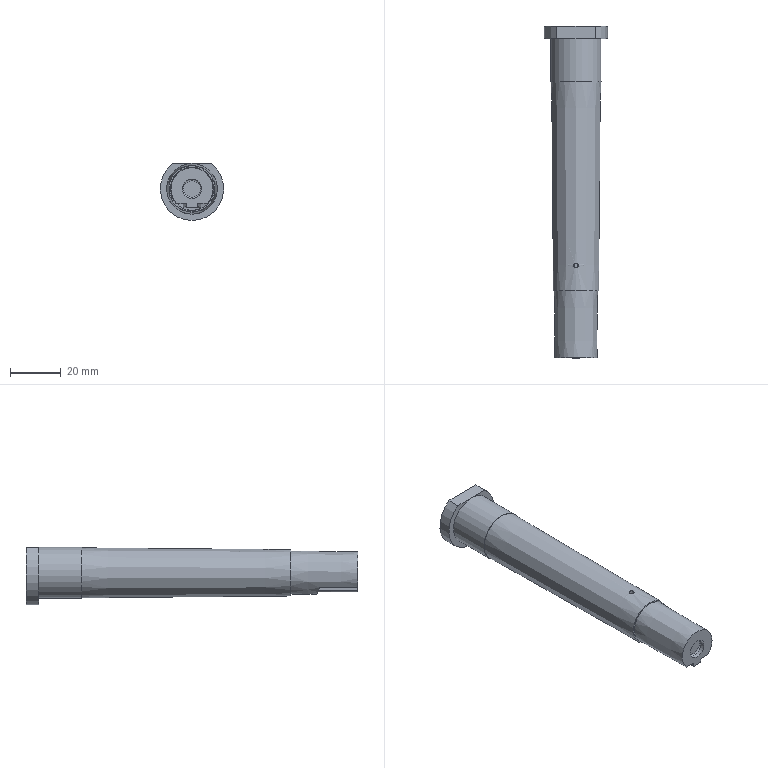Part | NX | features solid 2 | 1 solid | 31 faces | box 25 x 130.744 x 22.5 mm | volume 33270 mm3 | plane 14 | cylinder 9 | cone 4 | spline 2 | torus 2 | commonest cylinder face diameters 1 x2 7.537 x2 6 x1 9 x1 14 x1 20 x1
STEP:
#1=CARTESIAN_POINT('',(-7.5,132.,18.725));
#2=VERTEX_POINT('',#1);
#3=CARTESIAN_POINT('',(7.5,132.,18.725));
#4=VERTEX_POINT('',#3);
#5=CARTESIAN_POINT('',(0.,132.,18.725));
#6=DIRECTION('',(-1.,0.,0.));
#7=VECTOR('',#6,1000.);
#8=LINE('',#5,#7);
#9=EDGE_CURVE('',#2,#4,#8,.F.);
#10=ORIENTED_EDGE('',*,*,#9,.T.);
#11=CARTESIAN_POINT('',(0.,132.,8.725));
#12=DIRECTION('',(0.,1.,0.));
#13=DIRECTION('',(0.,0.,1.));
#14=AXIS2_PLACEMENT_3D('',#11,#12,#13);
#15=CIRCLE('',#14,12.5);
#16=EDGE_CURVE('',#4,#2,#15,.T.);
#17=ORIENTED_EDGE('',*,*,#16,.T.);
#18=EDGE_LOOP('',(#10,#17));
#19=FACE_BOUND('',#18,.T.);
#20=CARTESIAN_POINT('',(7.,132.,8.725));
#21=VERTEX_POINT('',#20);
#22=CARTESIAN_POINT('',(0.,132.,8.725));
#23=DIRECTION('',(0.,-1.,0.));
#24=DIRECTION('',(1.,0.,0.));
#25=AXIS2_PLACEMENT_3D('',#22,#23,#24);
#26=CIRCLE('',#25,7.);
#27=EDGE_CURVE('',#21,#21,#26,.T.);
#28=ORIENTED_EDGE('',*,*,#27,.T.);
#29=EDGE_LOOP('',(#28));
#30=FACE_BOUND('',#29,.T.);
#31=CARTESIAN_POINT('',(0.,132.,-5.275));
#32=DIRECTION('',(0.,1.,0.));
#33=DIRECTION('',(0.,0.,1.));
#34=AXIS2_PLACEMENT_3D('',#31,#32,#33);
#35=PLANE('',#34);
#36=ADVANCED_FACE('',(#19,#30),#35,.T.);
#37=CARTESIAN_POINT('',(6.03,1.256,3.004));
#38=VERTEX_POINT('',#37);
#39=CARTESIAN_POINT('',(2.188,1.256,3.004));
#40=VERTEX_POINT('',#39);
#41=CARTESIAN_POINT('',(0.,1.256,3.004));
#42=DIRECTION('',(-1.,0.,0.));
#43=VECTOR('',#42,1000.);
#44=LINE('',#41,#43);
#45=EDGE_CURVE('',#38,#40,#44,.T.);
#46=ORIENTED_EDGE('',*,*,#45,.T.);
#47=CARTESIAN_POINT('',(3.558,17.115,2.805));
#48=VERTEX_POINT('',#47);
#49=CARTESIAN_POINT('',(2.188,1.256,3.004));
#50=CARTESIAN_POINT('',(2.645,6.543,2.937));
#51=CARTESIAN_POINT('',(3.102,11.829,2.87));
#52=CARTESIAN_POINT('',(3.558,17.115,2.805));
#53=B_SPLINE_CURVE_WITH_KNOTS('',3,(#49,#50,#51,#52),.UNSPECIFIED.,.F.,.F.,(4,4),(0.,0.01592),.UNSPECIFIED.);
#54=EDGE_CURVE('',#40,#48,#53,.T.);
#55=ORIENTED_EDGE('',*,*,#54,.T.);
#56=CARTESIAN_POINT('',(6.03,16.408,2.813));
#57=VERTEX_POINT('',#56);
#58=CARTESIAN_POINT('',(3.558,17.115,2.805));
#59=CARTESIAN_POINT('',(4.399,16.941,2.807));
#60=CARTESIAN_POINT('',(5.223,16.705,2.81));
#61=CARTESIAN_POINT('',(6.03,16.408,2.813));
#62=B_SPLINE_CURVE_WITH_KNOTS('',3,(#58,#59,#60,#61),.UNSPECIFIED.,.F.,.F.,(4,4),(0.009661,0.0122),.UNSPECIFIED.);
#63=EDGE_CURVE('',#48,#57,#62,.T.);
#64=ORIENTED_EDGE('',*,*,#63,.T.);
#65=CARTESIAN_POINT('',(6.03,16.408,2.813));
#66=CARTESIAN_POINT('',(6.03,11.358,2.876));
#67=CARTESIAN_POINT('',(6.03,6.307,2.94));
#68=CARTESIAN_POINT('',(6.03,1.256,3.004));
#69=B_SPLINE_CURVE_WITH_KNOTS('',3,(#65,#66,#67,#68),.UNSPECIFIED.,.F.,.F.,(4,4),(0.,0.01515),.UNSPECIFIED.);
#70=EDGE_CURVE('',#57,#38,#69,.T.);
#71=ORIENTED_EDGE('',*,*,#70,.T.);
#72=EDGE_LOOP('',(#46,#55,#64,#71));
#73=FACE_BOUND('',#72,.T.);
#74=CARTESIAN_POINT('',(6.03,17.21,2.803));
#75=CARTESIAN_POINT('',(2.165,17.21,2.803));
#76=CARTESIAN_POINT('',(6.03,16.943,2.807));
#77=CARTESIAN_POINT('',(2.165,16.943,2.807));
#78=CARTESIAN_POINT('',(6.03,11.625,2.873));
#79=CARTESIAN_POINT('',(2.165,11.625,2.873));
#80=CARTESIAN_POINT('',(6.03,6.307,2.94));
#81=CARTESIAN_POINT('',(2.165,6.307,2.94));
#82=CARTESIAN_POINT('',(6.03,1.256,3.004));
#83=CARTESIAN_POINT('',(2.165,1.256,3.004));
#84=B_SPLINE_SURFACE_WITH_KNOTS('',3,1,((#74,#75),(#76,#77),(#78,#79),(#80,#81),(#82,#83)),.SURF_OF_LINEAR_EXTRUSION.,.F.,.F.,.F.,(4,1,4),(2,2),(-0.05294,0.,1.),(0.,0.3205),.UNSPECIFIED.);
#85=ADVANCED_FACE('',(#73),#84,.T.);
#86=CARTESIAN_POINT('',(-6.03,16.408,2.813));
#87=VERTEX_POINT('',#86);
#88=CARTESIAN_POINT('',(5.961,16.434,2.744));
#89=VERTEX_POINT('',#88);
#90=CARTESIAN_POINT('',(5.961,16.434,2.744));
#91=CARTESIAN_POINT('',(5.183,16.724,1.965));
#92=CARTESIAN_POINT('',(3.343,17.276,0.7218));
#93=CARTESIAN_POINT('',(-0.04988,17.621,0.03708));
#94=CARTESIAN_POINT('',(-3.426,17.259,0.7574));
#95=CARTESIAN_POINT('',(-5.261,16.698,2.025));
#96=CARTESIAN_POINT('',(-6.03,16.408,2.813));
#97=B_SPLINE_CURVE_WITH_KNOTS('',3,(#90,#91,#92,#93,#94,#95,#96),.UNSPECIFIED.,.F.,.F.,(4,1,1,1,4),(0.,0.00337,0.00674,0.01011,0.01348),.UNSPECIFIED.);
#98=EDGE_CURVE('',#87,#89,#97,.F.);
#99=ORIENTED_EDGE('',*,*,#98,.F.);
#100=CARTESIAN_POINT('',(-6.03,1.256,3.004));
#101=VERTEX_POINT('',#100);
#102=CARTESIAN_POINT('',(-6.03,1.256,3.004));
#103=CARTESIAN_POINT('',(-6.03,6.307,2.94));
#104=CARTESIAN_POINT('',(-6.03,11.358,2.876));
#105=CARTESIAN_POINT('',(-6.03,16.408,2.813));
#106=B_SPLINE_CURVE_WITH_KNOTS('',3,(#102,#103,#104,#105),.UNSPECIFIED.,.F.,.F.,(4,4),(0.,0.01515),.UNSPECIFIED.);
#107=EDGE_CURVE('',#101,#87,#106,.T.);
#108=ORIENTED_EDGE('',*,*,#107,.F.);
#109=CARTESIAN_POINT('',(0.,1.256,8.725));
#110=DIRECTION('',(0.,1.,0.));
#111=DIRECTION('',(-0.7254,0.,-0.6883));
#112=AXIS2_PLACEMENT_3D('',#109,#110,#111);
#113=CIRCLE('',#112,8.312);
#114=EDGE_CURVE('',#38,#101,#113,.F.);
#115=ORIENTED_EDGE('',*,*,#114,.F.);
#116=ORIENTED_EDGE('',*,*,#70,.F.);
#117=CARTESIAN_POINT('',(5.961,16.434,2.744));
#118=CARTESIAN_POINT('',(5.969,16.431,2.751));
#119=CARTESIAN_POINT('',(5.984,16.426,2.767));
#120=CARTESIAN_POINT('',(6.007,16.417,2.79));
#121=CARTESIAN_POINT('',(6.022,16.411,2.806));
#122=CARTESIAN_POINT('',(6.03,16.408,2.813));
#123=B_SPLINE_CURVE_WITH_KNOTS('',3,(#117,#118,#119,#120,#121,#122),.UNSPECIFIED.,.F.,.F.,(4,1,1,4),(0.,0.3333,0.6667,1.),.QUASI_UNIFORM_KNOTS.);
#124=EDGE_CURVE('',#89,#57,#123,.T.);
#125=ORIENTED_EDGE('',*,*,#124,.F.);
#126=EDGE_LOOP('',(#99,#108,#115,#116,#125));
#127=FACE_BOUND('',#126,.T.);
#128=CARTESIAN_POINT('',(0.,27.637,17.268));
#129=VERTEX_POINT('',#128);
#130=CARTESIAN_POINT('',(0.,27.637,8.725));
#131=DIRECTION('',(0.,1.,0.));
#132=DIRECTION('',(0.,0.,1.));
#133=AXIS2_PLACEMENT_3D('',#130,#131,#132);
#134=CIRCLE('',#133,8.543);
#135=EDGE_CURVE('',#129,#129,#134,.F.);
#136=ORIENTED_EDGE('',*,*,#135,.T.);
#137=EDGE_LOOP('',(#136));
#138=FACE_BOUND('',#137,.T.);
#139=CARTESIAN_POINT('',(0.,14.447,8.725));
#140=DIRECTION('',(0.,1.,0.));
#141=DIRECTION('',(0.,0.,-1.));
#142=AXIS2_PLACEMENT_3D('',#139,#140,#141);
#143=CONICAL_SURFACE('',#142,8.427,0.008727);
#144=ADVANCED_FACE('',(#127,#138),#143,.T.);
#145=CARTESIAN_POINT('',(0.,27.637,-0.3898));
#146=VERTEX_POINT('',#145);
#147=CARTESIAN_POINT('',(0.,27.637,8.725));
#148=DIRECTION('',(0.,-1.,0.));
#149=DIRECTION('',(0.,0.,-1.));
#150=AXIS2_PLACEMENT_3D('',#147,#148,#149);
#151=CIRCLE('',#150,9.115);
#152=EDGE_CURVE('',#146,#146,#151,.F.);
#153=ORIENTED_EDGE('',*,*,#152,.F.);
#154=EDGE_LOOP('',(#153));
#155=FACE_BOUND('',#154,.T.);
#156=ORIENTED_EDGE('',*,*,#135,.F.);
#157=EDGE_LOOP('',(#156));
#158=FACE_BOUND('',#157,.T.);
#159=CARTESIAN_POINT('',(0.,27.637,8.725));
#160=DIRECTION('',(0.,-1.,0.));
#161=DIRECTION('',(0.,0.,1.));
#162=AXIS2_PLACEMENT_3D('',#159,#160,#161);
#163=PLANE('',#162);
#164=ADVANCED_FACE('',(#155,#158),#163,.T.);
#165=ORIENTED_EDGE('',*,*,#152,.T.);
#166=EDGE_LOOP('',(#165));
#167=FACE_BOUND('',#166,.T.);
#168=CARTESIAN_POINT('',(0.,110.,-1.109));
#169=VERTEX_POINT('',#168);
#170=CARTESIAN_POINT('',(0.,110.,8.725));
#171=DIRECTION('',(0.,-1.,0.));
#172=DIRECTION('',(0.,0.,-1.));
#173=AXIS2_PLACEMENT_3D('',#170,#171,#172);
#174=CIRCLE('',#173,9.834);
#175=EDGE_CURVE('',#169,#169,#174,.F.);
#176=ORIENTED_EDGE('',*,*,#175,.F.);
#177=EDGE_LOOP('',(#176));
#178=FACE_BOUND('',#177,.T.);
#179=CARTESIAN_POINT('',(-0.9135,37.634,17.882));
#180=VERTEX_POINT('',#179);
#181=CARTESIAN_POINT('',(-0.7599,38.361,17.907));
#182=CARTESIAN_POINT('',(-1.012,37.629,17.871));
#183=CARTESIAN_POINT('',(-0.6747,36.928,17.902));
#184=CARTESIAN_POINT('',(0.05937,36.673,17.93));
#185=CARTESIAN_POINT('',(0.7563,37.011,17.895));
#186=CARTESIAN_POINT('',(1.107,38.004,17.865));
#187=CARTESIAN_POINT('',(0.1856,38.828,17.962));
#188=CARTESIAN_POINT('',(-0.7599,38.361,17.907));
#189=CARTESIAN_POINT('',(-1.012,37.629,17.871));
#190=CARTESIAN_POINT('',(-0.6747,36.928,17.902));
#191=B_SPLINE_CURVE_WITH_KNOTS('',3,(#181,#182,#183,#184,#185,#186,#187,#188,#189,#190),.UNSPECIFIED.,.T.,.F.,(1,1,1,1,1,1,1,1,1,1,1,1,1,1),(-0.002866,-0.001433,-0.0007165,0.,0.0007165,0.001433,0.00215,0.002866,0.004299,0.005016,0.005732,0.006449,0.007165,0.007882),.UNSPECIFIED.);
#192=EDGE_CURVE('',#180,#180,#191,.T.);
#193=ORIENTED_EDGE('',*,*,#192,.F.);
#194=EDGE_LOOP('',(#193));
#195=FACE_BOUND('',#194,.T.);
#196=CARTESIAN_POINT('',(0.,48.993,8.725));
#197=DIRECTION('',(0.,1.,0.));
#198=DIRECTION('',(0.,0.,-1.));
#199=AXIS2_PLACEMENT_3D('',#196,#197,#198);
#200=CONICAL_SURFACE('',#199,9.301,0.008727);
#201=ADVANCED_FACE('',(#167,#178,#195),#200,.T.);
#202=CARTESIAN_POINT('',(-3.769,1.256,8.725));
#203=VERTEX_POINT('',#202);
#204=CARTESIAN_POINT('',(3.769,1.256,8.725));
#205=VERTEX_POINT('',#204);
#206=CARTESIAN_POINT('',(0.,1.256,8.725));
#207=DIRECTION('',(0.,1.,0.));
#208=DIRECTION('',(-1.,0.,0.));
#209=AXIS2_PLACEMENT_3D('',#206,#207,#208);
#210=CIRCLE('',#209,3.769);
#211=EDGE_CURVE('',#203,#205,#210,.T.);
#212=ORIENTED_EDGE('',*,*,#211,.T.);
#213=CARTESIAN_POINT('',(0.,1.256,8.725));
#214=DIRECTION('',(0.,1.,0.));
#215=DIRECTION('',(1.,0.,0.));
#216=AXIS2_PLACEMENT_3D('',#213,#214,#215);
#217=CIRCLE('',#216,3.769);
#218=EDGE_CURVE('',#205,#203,#217,.T.);
#219=ORIENTED_EDGE('',*,*,#218,.T.);
#220=EDGE_LOOP('',(#212,#219));
#221=FACE_BOUND('',#220,.T.);
#222=CARTESIAN_POINT('',(-2.07,1.256,1.656));
#223=VERTEX_POINT('',#222);
#224=CARTESIAN_POINT('',(-2.188,1.256,3.004));
#225=VERTEX_POINT('',#224);
#226=CARTESIAN_POINT('',(-2.03,1.256,1.2));
#227=DIRECTION('',(-0.08749,0.,0.9962));
#228=VECTOR('',#227,1000.);
#229=LINE('',#226,#228);
#230=EDGE_CURVE('',#223,#225,#229,.T.);
#231=ORIENTED_EDGE('',*,*,#230,.F.);
#232=CARTESIAN_POINT('',(-1.57,1.256,1.2));
#233=VERTEX_POINT('',#232);
#234=CARTESIAN_POINT('',(-1.57,1.256,1.7));
#235=DIRECTION('',(0.,1.,0.));
#236=DIRECTION('',(1.,0.,0.));
#237=AXIS2_PLACEMENT_3D('',#234,#235,#236);
#238=ELLIPSE('',#237,0.5019,0.5);
#239=EDGE_CURVE('',#223,#233,#238,.F.);
#240=ORIENTED_EDGE('',*,*,#239,.T.);
#241=CARTESIAN_POINT('',(1.57,1.256,1.2));
#242=VERTEX_POINT('',#241);
#243=CARTESIAN_POINT('',(0.,1.256,1.2));
#244=DIRECTION('',(1.,0.,0.));
#245=VECTOR('',#244,1000.);
#246=LINE('',#243,#245);
#247=EDGE_CURVE('',#233,#242,#246,.T.);
#248=ORIENTED_EDGE('',*,*,#247,.T.);
#249=CARTESIAN_POINT('',(2.07,1.256,1.656));
#250=VERTEX_POINT('',#249);
#251=CARTESIAN_POINT('',(1.57,1.256,1.7));
#252=DIRECTION('',(0.,1.,0.));
#253=DIRECTION('',(1.,0.,0.));
#254=AXIS2_PLACEMENT_3D('',#251,#252,#253);
#255=ELLIPSE('',#254,0.5019,0.5);
#256=EDGE_CURVE('',#242,#250,#255,.F.);
#257=ORIENTED_EDGE('',*,*,#256,.T.);
#258=CARTESIAN_POINT('',(1.997,1.256,0.8247));
#259=DIRECTION('',(0.08749,0.,0.9962));
#260=VECTOR('',#259,1000.);
#261=LINE('',#258,#260);
#262=EDGE_CURVE('',#250,#40,#261,.T.);
#263=ORIENTED_EDGE('',*,*,#262,.T.);
#264=ORIENTED_EDGE('',*,*,#45,.F.);
#265=ORIENTED_EDGE('',*,*,#114,.T.);
#266=CARTESIAN_POINT('',(0.,1.256,3.004));
#267=DIRECTION('',(-1.,0.,0.));
#268=VECTOR('',#267,1000.);
#269=LINE('',#266,#268);
#270=EDGE_CURVE('',#225,#101,#269,.T.);
#271=ORIENTED_EDGE('',*,*,#270,.F.);
#272=EDGE_LOOP('',(#231,#240,#248,#257,#263,#264,#265,#271));
#273=FACE_BOUND('',#272,.T.);
#274=CARTESIAN_POINT('',(-18.15,1.256,17.77));
#275=DIRECTION('',(0.,1.,0.));
#276=DIRECTION('',(-1.,0.,0.));
#277=AXIS2_PLACEMENT_3D('',#274,#275,#276);
#278=PLANE('',#277);
#279=ADVANCED_FACE('',(#221,#273),#278,.F.);
#280=CARTESIAN_POINT('',(-3.558,17.115,2.805));
#281=VERTEX_POINT('',#280);
#282=CARTESIAN_POINT('',(-6.03,16.408,2.813));
#283=CARTESIAN_POINT('',(-5.217,16.707,2.81));
#284=CARTESIAN_POINT('',(-4.393,16.942,2.807));
#285=CARTESIAN_POINT('',(-3.558,17.115,2.805));
#286=B_SPLINE_CURVE_WITH_KNOTS('',3,(#282,#283,#284,#285),.UNSPECIFIED.,.F.,.F.,(4,4),(0.,0.002557),.UNSPECIFIED.);
#287=EDGE_CURVE('',#87,#281,#286,.T.);
#288=ORIENTED_EDGE('',*,*,#287,.T.);
#289=CARTESIAN_POINT('',(-3.558,17.115,2.805));
#290=CARTESIAN_POINT('',(-3.102,11.829,2.87));
#291=CARTESIAN_POINT('',(-2.645,6.543,2.937));
#292=CARTESIAN_POINT('',(-2.188,1.256,3.004));
#293=B_SPLINE_CURVE_WITH_KNOTS('',3,(#289,#290,#291,#292),.UNSPECIFIED.,.F.,.F.,(4,4),(0.0003674,0.01629),.UNSPECIFIED.);
#294=EDGE_CURVE('',#281,#225,#293,.T.);
#295=ORIENTED_EDGE('',*,*,#294,.T.);
#296=ORIENTED_EDGE('',*,*,#270,.T.);
#297=ORIENTED_EDGE('',*,*,#107,.T.);
#298=EDGE_LOOP('',(#288,#295,#296,#297));
#299=FACE_BOUND('',#298,.T.);
#300=CARTESIAN_POINT('',(-2.165,17.21,2.803));
#301=CARTESIAN_POINT('',(-6.03,17.21,2.803));
#302=CARTESIAN_POINT('',(-2.165,16.943,2.807));
#303=CARTESIAN_POINT('',(-6.03,16.943,2.807));
#304=CARTESIAN_POINT('',(-2.165,11.625,2.873));
#305=CARTESIAN_POINT('',(-6.03,11.625,2.873));
#306=CARTESIAN_POINT('',(-2.165,6.307,2.94));
#307=CARTESIAN_POINT('',(-6.03,6.307,2.94));
#308=CARTESIAN_POINT('',(-2.165,1.256,3.004));
#309=CARTESIAN_POINT('',(-6.03,1.256,3.004));
#310=B_SPLINE_SURFACE_WITH_KNOTS('',3,1,((#300,#301),(#302,#303),(#304,#305),(#306,#307),(#308,#309)),.SURF_OF_LINEAR_EXTRUSION.,.F.,.F.,.F.,(4,1,4),(2,2),(-0.05294,0.,1.),(0.6795,1.),.UNSPECIFIED.);
#311=ADVANCED_FACE('',(#299),#310,.T.);
#312=CARTESIAN_POINT('',(3.46,17.146,1.656));
#313=VERTEX_POINT('',#312);
#314=CARTESIAN_POINT('',(-1.775,0.1553,-41.03));
#315=DIRECTION('',(0.9924,-0.08682,-0.08716));
#316=DIRECTION('',(-0.08682,0.007596,-0.9962));
#317=AXIS2_PLACEMENT_3D('',#314,#315,#316);
#318=ELLIPSE('',#317,204.965,17.775);
#319=EDGE_CURVE('',#313,#48,#318,.T.);
#320=ORIENTED_EDGE('',*,*,#319,.F.);
#321=CARTESIAN_POINT('',(2.969,17.242,1.2));
#322=VERTEX_POINT('',#321);
#323=CARTESIAN_POINT('',(3.46,17.146,1.656));
#324=CARTESIAN_POINT('',(3.439,17.152,1.407));
#325=CARTESIAN_POINT('',(3.215,17.199,1.2));
#326=CARTESIAN_POINT('',(2.969,17.242,1.2));
#327=B_SPLINE_CURVE_WITH_KNOTS('',3,(#323,#324,#325,#326),.UNSPECIFIED.,.F.,.F.,(4,4),(0.,0.0007397),.UNSPECIFIED.);
#328=EDGE_CURVE('',#313,#322,#327,.T.);
#329=ORIENTED_EDGE('',*,*,#328,.T.);
#330=CARTESIAN_POINT('',(-2.969,17.242,1.2));
#331=VERTEX_POINT('',#330);
#332=CARTESIAN_POINT('',(0.,0.,1.2));
#333=DIRECTION('',(0.,0.,-1.));
#334=DIRECTION('',(-1.,0.,0.));
#335=AXIS2_PLACEMENT_3D('',#332,#333,#334);
#336=CIRCLE('',#335,17.495);
#337=EDGE_CURVE('',#331,#322,#336,.T.);
#338=ORIENTED_EDGE('',*,*,#337,.F.);
#339=CARTESIAN_POINT('',(-3.46,17.146,1.656));
#340=VERTEX_POINT('',#339);
#341=CARTESIAN_POINT('',(-2.969,17.242,1.2));
#342=CARTESIAN_POINT('',(-3.215,17.199,1.2));
#343=CARTESIAN_POINT('',(-3.439,17.152,1.407));
#344=CARTESIAN_POINT('',(-3.46,17.146,1.656));
#345=B_SPLINE_CURVE_WITH_KNOTS('',3,(#341,#342,#343,#344),.UNSPECIFIED.,.F.,.F.,(4,4),(0.,0.0007398),.UNSPECIFIED.);
#346=EDGE_CURVE('',#331,#340,#345,.T.);
#347=ORIENTED_EDGE('',*,*,#346,.T.);
#348=CARTESIAN_POINT('',(1.775,0.1553,-41.03));
#349=DIRECTION('',(-0.9924,-0.08682,-0.08716));
#350=DIRECTION('',(0.08682,0.007596,-0.9962));
#351=AXIS2_PLACEMENT_3D('',#348,#349,#350);
#352=ELLIPSE('',#351,204.965,17.775);
#353=EDGE_CURVE('',#281,#340,#352,.T.);
#354=ORIENTED_EDGE('',*,*,#353,.F.);
#355=ORIENTED_EDGE('',*,*,#287,.F.);
#356=ORIENTED_EDGE('',*,*,#98,.T.);
#357=ORIENTED_EDGE('',*,*,#124,.T.);
#358=ORIENTED_EDGE('',*,*,#63,.F.);
#359=EDGE_LOOP('',(#320,#329,#338,#347,#354,#355,#356,#357,#358));
#360=FACE_BOUND('',#359,.T.);
#361=CARTESIAN_POINT('',(0.,0.,4.707));
#362=DIRECTION('',(0.,0.,-1.));
#363=DIRECTION('',(1.,0.,0.));
#364=AXIS2_PLACEMENT_3D('',#361,#362,#363);
#365=CONICAL_SURFACE('',#364,17.465,0.008727);
#366=ADVANCED_FACE('',(#360),#365,.F.);
#367=CARTESIAN_POINT('',(-3.769,2.764,8.725));
#368=VERTEX_POINT('',#367);
#369=CARTESIAN_POINT('',(-3.769,1.256,8.725));
#370=DIRECTION('',(0.,1.,-0.000000008));
#371=VECTOR('',#370,1000.);
#372=LINE('',#369,#371);
#373=EDGE_CURVE('',#203,#368,#372,.T.);
#374=ORIENTED_EDGE('',*,*,#373,.T.);
#375=CARTESIAN_POINT('',(3.769,2.764,8.725));
#376=VERTEX_POINT('',#375);
#377=CARTESIAN_POINT('',(0.,2.764,8.725));
#378=DIRECTION('',(0.,1.,0.));
#379=DIRECTION('',(-1.,0.,0.));
#380=AXIS2_PLACEMENT_3D('',#377,#378,#379);
#381=CIRCLE('',#380,3.769);
#382=EDGE_CURVE('',#376,#368,#381,.F.);
#383=ORIENTED_EDGE('',*,*,#382,.F.);
#384=CARTESIAN_POINT('',(3.769,1.256,8.725));
#385=DIRECTION('',(0.,1.,0.000000008));
#386=VECTOR('',#385,1000.);
#387=LINE('',#384,#386);
#388=EDGE_CURVE('',#376,#205,#387,.F.);
#389=ORIENTED_EDGE('',*,*,#388,.T.);
#390=ORIENTED_EDGE('',*,*,#211,.F.);
#391=EDGE_LOOP('',(#374,#383,#389,#390));
#392=FACE_BOUND('',#391,.T.);
#393=CARTESIAN_POINT('',(0.,1.256,8.725));
#394=DIRECTION('',(0.,1.,0.));
#395=DIRECTION('',(1.,0.,0.));
#396=AXIS2_PLACEMENT_3D('',#393,#394,#395);
#397=CYLINDRICAL_SURFACE('',#396,3.769);
#398=ADVANCED_FACE('',(#392),#397,.F.);
#399=CARTESIAN_POINT('',(-3.266,3.266,8.725));
#400=VERTEX_POINT('',#399);
#401=CARTESIAN_POINT('',(-3.266,2.764,8.725));
#402=DIRECTION('',(0.,0.,1.));
#403=DIRECTION('',(0.,1.,0.));
#404=AXIS2_PLACEMENT_3D('',#401,#402,#403);
#405=CIRCLE('',#404,0.5025);
#406=EDGE_CURVE('',#368,#400,#405,.F.);
#407=ORIENTED_EDGE('',*,*,#406,.T.);
#408=CARTESIAN_POINT('',(3.266,3.266,8.725));
#409=VERTEX_POINT('',#408);
#410=CARTESIAN_POINT('',(0.,3.266,8.725));
#411=DIRECTION('',(0.,1.,0.));
#412=DIRECTION('',(-1.,0.,0.));
#413=AXIS2_PLACEMENT_3D('',#410,#411,#412);
#414=CIRCLE('',#413,3.266);
#415=EDGE_CURVE('',#409,#400,#414,.F.);
#416=ORIENTED_EDGE('',*,*,#415,.F.);
#417=CARTESIAN_POINT('',(3.266,2.764,8.725));
#418=DIRECTION('',(0.,0.,-1.));
#419=DIRECTION('',(0.,1.,0.));
#420=AXIS2_PLACEMENT_3D('',#417,#418,#419);
#421=CIRCLE('',#420,0.5025);
#422=EDGE_CURVE('',#409,#376,#421,.T.);
#423=ORIENTED_EDGE('',*,*,#422,.T.);
#424=ORIENTED_EDGE('',*,*,#382,.T.);
#425=EDGE_LOOP('',(#407,#416,#423,#424));
#426=FACE_BOUND('',#425,.T.);
#427=CARTESIAN_POINT('',(0.,2.764,8.725));
#428=DIRECTION('',(0.,1.,0.));
#429=DIRECTION('',(0.997,0.,0.07682));
#430=AXIS2_PLACEMENT_3D('',#427,#428,#429);
#431=TOROIDAL_SURFACE('',#430,3.266,0.5025);
#432=ADVANCED_FACE('',(#426),#431,.F.);
#433=ORIENTED_EDGE('',*,*,#422,.F.);
#434=CARTESIAN_POINT('',(0.,3.266,8.725));
#435=DIRECTION('',(0.,1.,0.));
#436=DIRECTION('',(1.,0.,0.));
#437=AXIS2_PLACEMENT_3D('',#434,#435,#436);
#438=CIRCLE('',#437,3.266);
#439=EDGE_CURVE('',#400,#409,#438,.F.);
#440=ORIENTED_EDGE('',*,*,#439,.F.);
#441=ORIENTED_EDGE('',*,*,#406,.F.);
#442=CARTESIAN_POINT('',(0.,2.764,8.725));
#443=DIRECTION('',(0.,1.,0.));
#444=DIRECTION('',(1.,0.,0.));
#445=AXIS2_PLACEMENT_3D('',#442,#443,#444);
#446=CIRCLE('',#445,3.769);
#447=EDGE_CURVE('',#368,#376,#446,.F.);
#448=ORIENTED_EDGE('',*,*,#447,.T.);
#449=EDGE_LOOP('',(#433,#440,#441,#448));
#450=FACE_BOUND('',#449,.T.);
#451=CARTESIAN_POINT('',(0.,2.764,8.725));
#452=DIRECTION('',(0.,1.,0.));
#453=DIRECTION('',(-0.997,0.,-0.07682));
#454=AXIS2_PLACEMENT_3D('',#451,#452,#453);
#455=TOROIDAL_SURFACE('',#454,3.266,0.5025);
#456=ADVANCED_FACE('',(#450),#455,.F.);
#457=ORIENTED_EDGE('',*,*,#388,.F.);
#458=ORIENTED_EDGE('',*,*,#447,.F.);
#459=ORIENTED_EDGE('',*,*,#373,.F.);
#460=ORIENTED_EDGE('',*,*,#218,.F.);
#461=EDGE_LOOP('',(#457,#458,#459,#460));
#462=FACE_BOUND('',#461,.T.);
#463=CARTESIAN_POINT('',(0.,1.256,8.725));
#464=DIRECTION('',(0.,1.,0.));
#465=DIRECTION('',(1.,0.,0.));
#466=AXIS2_PLACEMENT_3D('',#463,#464,#465);
#467=CYLINDRICAL_SURFACE('',#466,3.769);
#468=ADVANCED_FACE('',(#462),#467,.F.);
#469=ORIENTED_EDGE('',*,*,#415,.T.);
#470=ORIENTED_EDGE('',*,*,#439,.T.);
#471=EDGE_LOOP('',(#469,#470));
#472=FACE_BOUND('',#471,.T.);
#473=CARTESIAN_POINT('',(0.7538,3.266,1.188));
#474=DIRECTION('',(0.,1.,0.));
#475=DIRECTION('',(0.,0.,1.));
#476=AXIS2_PLACEMENT_3D('',#473,#474,#475);
#477=PLANE('',#476);
#478=ADVANCED_FACE('',(#472),#477,.F.);
#479=ORIENTED_EDGE('',*,*,#262,.F.);
#480=CARTESIAN_POINT('',(2.07,1.253,1.656));
#481=DIRECTION('',(0.08716,0.9962,0.));
#482=VECTOR('',#481,1000.);
#483=LINE('',#480,#482);
#484=EDGE_CURVE('',#250,#313,#483,.T.);
#485=ORIENTED_EDGE('',*,*,#484,.T.);
#486=ORIENTED_EDGE('',*,*,#319,.T.);
#487=ORIENTED_EDGE('',*,*,#54,.F.);
#488=EDGE_LOOP('',(#479,#485,#486,#487));
#489=FACE_BOUND('',#488,.T.);
#490=CARTESIAN_POINT('',(2.03,1.256,1.2));
#491=DIRECTION('',(0.9924,-0.08682,-0.08716));
#492=DIRECTION('',(-0.08749,0.,-0.9962));
#493=AXIS2_PLACEMENT_3D('',#490,#491,#492);
#494=PLANE('',#493);
#495=ADVANCED_FACE('',(#489),#494,.T.);
#496=ORIENTED_EDGE('',*,*,#353,.T.);
#497=CARTESIAN_POINT('',(-2.07,1.253,1.656));
#498=DIRECTION('',(0.08716,-0.9962,0.));
#499=VECTOR('',#498,1000.);
#500=LINE('',#497,#499);
#501=EDGE_CURVE('',#340,#223,#500,.T.);
#502=ORIENTED_EDGE('',*,*,#501,.T.);
#503=ORIENTED_EDGE('',*,*,#230,.T.);
#504=ORIENTED_EDGE('',*,*,#294,.F.);
#505=EDGE_LOOP('',(#496,#502,#503,#504));
#506=FACE_BOUND('',#505,.T.);
#507=CARTESIAN_POINT('',(-2.03,1.256,1.2));
#508=DIRECTION('',(-0.9924,-0.08682,-0.08716));
#509=DIRECTION('',(-0.08749,0.,0.9962));
#510=AXIS2_PLACEMENT_3D('',#507,#508,#509);
#511=PLANE('',#510);
#512=ADVANCED_FACE('',(#506),#511,.T.);
#513=ORIENTED_EDGE('',*,*,#247,.F.);
#514=CARTESIAN_POINT('',(-2.263,9.171,1.2));
#515=DIRECTION('',(0.08716,-0.9962,0.));
#516=VECTOR('',#515,1000.);
#517=LINE('',#514,#516);
#518=EDGE_CURVE('',#233,#331,#517,.F.);
#519=ORIENTED_EDGE('',*,*,#518,.T.);
#520=ORIENTED_EDGE('',*,*,#337,.T.);
#521=CARTESIAN_POINT('',(2.263,9.171,1.2));
#522=DIRECTION('',(0.08716,0.9962,0.));
#523=VECTOR('',#522,1000.);
#524=LINE('',#521,#523);
#525=EDGE_CURVE('',#322,#242,#524,.F.);
#526=ORIENTED_EDGE('',*,*,#525,.T.);
#527=EDGE_LOOP('',(#513,#519,#520,#526));
#528=FACE_BOUND('',#527,.T.);
#529=CARTESIAN_POINT('',(0.,9.369,1.2));
#530=DIRECTION('',(0.,0.,-1.));
#531=DIRECTION('',(-1.,0.,0.));
#532=AXIS2_PLACEMENT_3D('',#529,#530,#531);
#533=PLANE('',#532);
#534=ADVANCED_FACE('',(#528),#533,.T.);
#535=ORIENTED_EDGE('',*,*,#346,.F.);
#536=ORIENTED_EDGE('',*,*,#518,.F.);
#537=ORIENTED_EDGE('',*,*,#239,.F.);
#538=ORIENTED_EDGE('',*,*,#501,.F.);
#539=EDGE_LOOP('',(#535,#536,#537,#538));
#540=FACE_BOUND('',#539,.T.);
#541=CARTESIAN_POINT('',(-1.574,1.296,1.7));
#542=DIRECTION('',(0.08716,-0.9962,0.));
#543=DIRECTION('',(0.9962,0.08716,0.));
#544=AXIS2_PLACEMENT_3D('',#541,#542,#543);
#545=CYLINDRICAL_SURFACE('',#544,0.5);
#546=ADVANCED_FACE('',(#540),#545,.T.);
#547=ORIENTED_EDGE('',*,*,#256,.F.);
#548=ORIENTED_EDGE('',*,*,#525,.F.);
#549=ORIENTED_EDGE('',*,*,#328,.F.);
#550=ORIENTED_EDGE('',*,*,#484,.F.);
#551=EDGE_LOOP('',(#547,#548,#549,#550));
#552=FACE_BOUND('',#551,.T.);
#553=CARTESIAN_POINT('',(1.574,1.296,1.7));
#554=DIRECTION('',(0.08716,0.9962,0.));
#555=DIRECTION('',(-0.9962,0.08716,0.));
#556=AXIS2_PLACEMENT_3D('',#553,#554,#555);
#557=CYLINDRICAL_SURFACE('',#556,0.5);
#558=ADVANCED_FACE('',(#552),#557,.T.);
#559=CARTESIAN_POINT('',(0.,127.,18.725));
#560=VERTEX_POINT('',#559);
#561=CARTESIAN_POINT('',(0.,127.,8.725));
#562=DIRECTION('',(0.,1.,0.));
#563=DIRECTION('',(0.,0.,1.));
#564=AXIS2_PLACEMENT_3D('',#561,#562,#563);
#565=CIRCLE('',#564,10.);
#566=EDGE_CURVE('',#560,#560,#565,.F.);
#567=ORIENTED_EDGE('',*,*,#566,.T.);
#568=EDGE_LOOP('',(#567));
#569=FACE_BOUND('',#568,.T.);
#570=CARTESIAN_POINT('',(0.,110.,-1.275));
#571=VERTEX_POINT('',#570);
#572=CARTESIAN_POINT('',(0.,110.,8.725));
#573=DIRECTION('',(0.,-1.,0.));
#574=DIRECTION('',(0.,0.,-1.));
#575=AXIS2_PLACEMENT_3D('',#572,#573,#574);
#576=CIRCLE('',#575,10.);
#577=EDGE_CURVE('',#571,#571,#576,.F.);
#578=ORIENTED_EDGE('',*,*,#577,.T.);
#579=EDGE_LOOP('',(#578));
#580=FACE_BOUND('',#579,.T.);
#581=CARTESIAN_POINT('',(0.,125.625,8.725));
#582=DIRECTION('',(0.,-1.,0.));
#583=DIRECTION('',(0.,0.,-1.));
#584=AXIS2_PLACEMENT_3D('',#581,#582,#583);
#585=CYLINDRICAL_SURFACE('',#584,10.);
#586=ADVANCED_FACE('',(#569,#580),#585,.T.);
#587=CARTESIAN_POINT('',(7.5,127.,18.725));
#588=VERTEX_POINT('',#587);
#589=CARTESIAN_POINT('',(-7.5,127.,18.725));
#590=VERTEX_POINT('',#589);
#591=CARTESIAN_POINT('',(0.,127.,8.725));
#592=DIRECTION('',(0.,1.,0.));
#593=DIRECTION('',(0.,0.,1.));
#594=AXIS2_PLACEMENT_3D('',#591,#592,#593);
#595=CIRCLE('',#594,12.5);
#596=EDGE_CURVE('',#588,#590,#595,.T.);
#597=ORIENTED_EDGE('',*,*,#596,.F.);
#598=CARTESIAN_POINT('',(0.,127.,18.725));
#599=DIRECTION('',(-1.,0.,0.));
#600=VECTOR('',#599,1000.);
#601=LINE('',#598,#600);
#602=EDGE_CURVE('',#560,#588,#601,.F.);
#603=ORIENTED_EDGE('',*,*,#602,.F.);
#604=ORIENTED_EDGE('',*,*,#566,.F.);
#605=CARTESIAN_POINT('',(0.,127.,18.725));
#606=DIRECTION('',(-1.,0.,0.));
#607=VECTOR('',#606,1000.);
#608=LINE('',#605,#607);
#609=EDGE_CURVE('',#590,#560,#608,.F.);
#610=ORIENTED_EDGE('',*,*,#609,.F.);
#611=EDGE_LOOP('',(#597,#603,#604,#610));
#612=FACE_BOUND('',#611,.T.);
#613=CARTESIAN_POINT('',(0.,127.,8.725));
#614=DIRECTION('',(0.,1.,0.));
#615=DIRECTION('',(0.,0.,1.));
#616=AXIS2_PLACEMENT_3D('',#613,#614,#615);
#617=PLANE('',#616);
#618=ADVANCED_FACE('',(#612),#617,.F.);
#619=CARTESIAN_POINT('',(-7.5,124.,18.725));
#620=DIRECTION('',(0.,1.,0.));
#621=VECTOR('',#620,1000.);
#622=LINE('',#619,#621);
#623=EDGE_CURVE('',#590,#2,#622,.T.);
#624=ORIENTED_EDGE('',*,*,#623,.T.);
#625=ORIENTED_EDGE('',*,*,#16,.F.);
#626=CARTESIAN_POINT('',(7.5,124.,18.725));
#627=DIRECTION('',(0.,1.,0.));
#628=VECTOR('',#627,1000.);
#629=LINE('',#626,#628);
#630=EDGE_CURVE('',#4,#588,#629,.F.);
#631=ORIENTED_EDGE('',*,*,#630,.T.);
#632=ORIENTED_EDGE('',*,*,#596,.T.);
#633=EDGE_LOOP('',(#624,#625,#631,#632));
#634=FACE_BOUND('',#633,.T.);
#635=CARTESIAN_POINT('',(0.,124.,8.725));
#636=DIRECTION('',(0.,1.,0.));
#637=DIRECTION('',(0.,0.,1.));
#638=AXIS2_PLACEMENT_3D('',#635,#636,#637);
#639=CYLINDRICAL_SURFACE('',#638,12.5);
#640=ADVANCED_FACE('',(#634),#639,.T.);
#641=ORIENTED_EDGE('',*,*,#175,.T.);
#642=EDGE_LOOP('',(#641));
#643=FACE_BOUND('',#642,.T.);
#644=ORIENTED_EDGE('',*,*,#577,.F.);
#645=EDGE_LOOP('',(#644));
#646=FACE_BOUND('',#645,.T.);
#647=CARTESIAN_POINT('',(0.,110.,8.725));
#648=DIRECTION('',(0.,-1.,0.));
#649=DIRECTION('',(0.,0.,-1.));
#650=AXIS2_PLACEMENT_3D('',#647,#648,#649);
#651=PLANE('',#650);
#652=ADVANCED_FACE('',(#643,#646),#651,.T.);
#653=ORIENTED_EDGE('',*,*,#602,.T.);
#654=ORIENTED_EDGE('',*,*,#630,.F.);
#655=ORIENTED_EDGE('',*,*,#9,.F.);
#656=ORIENTED_EDGE('',*,*,#623,.F.);
#657=ORIENTED_EDGE('',*,*,#609,.T.);
#658=EDGE_LOOP('',(#653,#654,#655,#656,#657));
#659=FACE_BOUND('',#658,.T.);
#660=CARTESIAN_POINT('',(0.,127.,18.725));
#661=DIRECTION('',(0.,0.,-1.));
#662=DIRECTION('',(0.,1.,0.));
#663=AXIS2_PLACEMENT_3D('',#660,#661,#662);
#664=PLANE('',#663);
#665=ADVANCED_FACE('',(#659),#664,.F.);
#666=CARTESIAN_POINT('',(-0.7554,37.688,14.836));
#667=VERTEX_POINT('',#666);
#668=CARTESIAN_POINT('',(0.,37.688,14.836));
#669=DIRECTION('',(0.,0.,-1.));
#670=DIRECTION('',(-1.,0.,0.));
#671=AXIS2_PLACEMENT_3D('',#668,#669,#670);
#672=CIRCLE('',#671,0.7554);
#673=EDGE_CURVE('',#667,#667,#672,.T.);
#674=ORIENTED_EDGE('',*,*,#673,.F.);
#675=EDGE_LOOP('',(#674));
#676=FACE_BOUND('',#675,.T.);
#677=CARTESIAN_POINT('',(0.,37.688,14.836));
#678=DIRECTION('',(0.,0.,-1.));
#679=DIRECTION('',(-1.,0.,0.));
#680=AXIS2_PLACEMENT_3D('',#677,#678,#679);
#681=PLANE('',#680);
#682=ADVANCED_FACE('',(#676),#681,.F.);
#683=ORIENTED_EDGE('',*,*,#673,.T.);
#684=EDGE_LOOP('',(#683));
#685=FACE_BOUND('',#684,.T.);
#686=ORIENTED_EDGE('',*,*,#192,.T.);
#687=EDGE_LOOP('',(#686));
#688=FACE_BOUND('',#687,.T.);
#689=CARTESIAN_POINT('',(0.,37.688,15.336));
#690=DIRECTION('',(0.,0.,1.));
#691=DIRECTION('',(-1.,0.,0.));
#692=AXIS2_PLACEMENT_3D('',#689,#690,#691);
#693=CONICAL_SURFACE('',#692,0.7816,0.05236);
#694=ADVANCED_FACE('',(#685,#688),#693,.F.);
#695=CARTESIAN_POINT('',(7.,130.6,8.725));
#696=VERTEX_POINT('',#695);
#697=CARTESIAN_POINT('',(0.,130.6,8.725));
#698=DIRECTION('',(0.,1.,0.));
#699=DIRECTION('',(1.,0.,0.));
#700=AXIS2_PLACEMENT_3D('',#697,#698,#699);
#701=CIRCLE('',#700,7.);
#702=EDGE_CURVE('',#696,#696,#701,.F.);
#703=ORIENTED_EDGE('',*,*,#702,.F.);
#704=EDGE_LOOP('',(#703));
#705=FACE_BOUND('',#704,.T.);
#706=CARTESIAN_POINT('',(4.5,130.6,8.725));
#707=VERTEX_POINT('',#706);
#708=CARTESIAN_POINT('',(0.,130.6,8.725));
#709=DIRECTION('',(0.,1.,0.));
#710=DIRECTION('',(1.,0.,0.));
#711=AXIS2_PLACEMENT_3D('',#708,#709,#710);
#712=CIRCLE('',#711,4.5);
#713=EDGE_CURVE('',#707,#707,#712,.F.);
#714=ORIENTED_EDGE('',*,*,#713,.T.);
#715=EDGE_LOOP('',(#714));
#716=FACE_BOUND('',#715,.T.);
#717=CARTESIAN_POINT('',(0.,130.6,8.725));
#718=DIRECTION('',(0.,-1.,0.));
#719=DIRECTION('',(0.,0.,-1.));
#720=AXIS2_PLACEMENT_3D('',#717,#718,#719);
#721=PLANE('',#720);
#722=ADVANCED_FACE('',(#705,#716),#721,.F.);
#723=ORIENTED_EDGE('',*,*,#702,.T.);
#724=EDGE_LOOP('',(#723));
#725=FACE_BOUND('',#724,.T.);
#726=ORIENTED_EDGE('',*,*,#27,.F.);
#727=EDGE_LOOP('',(#726));
#728=FACE_BOUND('',#727,.T.);
#729=CARTESIAN_POINT('',(0.,132.,8.725));
#730=DIRECTION('',(0.,-1.,0.));
#731=DIRECTION('',(1.,0.,0.));
#732=AXIS2_PLACEMENT_3D('',#729,#730,#731);
#733=CYLINDRICAL_SURFACE('',#732,7.);
#734=ADVANCED_FACE('',(#725,#728),#733,.F.);
#735=ORIENTED_EDGE('',*,*,#713,.F.);
#736=EDGE_LOOP('',(#735));
#737=FACE_BOUND('',#736,.T.);
#738=CARTESIAN_POINT('',(4.5,132.,8.725));
#739=VERTEX_POINT('',#738);
#740=CARTESIAN_POINT('',(0.,132.,8.725));
#741=DIRECTION('',(0.,-1.,0.));
#742=DIRECTION('',(1.,0.,0.));
#743=AXIS2_PLACEMENT_3D('',#740,#741,#742);
#744=CIRCLE('',#743,4.5);
#745=EDGE_CURVE('',#739,#739,#744,.T.);
#746=ORIENTED_EDGE('',*,*,#745,.T.);
#747=EDGE_LOOP('',(#746));
#748=FACE_BOUND('',#747,.T.);
#749=CARTESIAN_POINT('',(0.,132.,8.725));
#750=DIRECTION('',(0.,-1.,0.));
#751=DIRECTION('',(1.,0.,0.));
#752=AXIS2_PLACEMENT_3D('',#749,#750,#751);
#753=CYLINDRICAL_SURFACE('',#752,4.5);
#754=ADVANCED_FACE('',(#737,#748),#753,.T.);
#755=CARTESIAN_POINT('',(0.,22.,5.725));
#756=VERTEX_POINT('',#755);
#757=CARTESIAN_POINT('',(0.,22.,8.725));
#758=DIRECTION('',(0.,-1.,0.));
#759=DIRECTION('',(0.,0.,-1.));
#760=AXIS2_PLACEMENT_3D('',#757,#758,#759);
#761=CIRCLE('',#760,3.);
#762=EDGE_CURVE('',#756,#756,#761,.F.);
#763=ORIENTED_EDGE('',*,*,#762,.T.);
#764=EDGE_LOOP('',(#763));
#765=FACE_BOUND('',#764,.T.);
#766=CARTESIAN_POINT('',(0.,22.,8.725));
#767=DIRECTION('',(0.,-1.,0.));
#768=DIRECTION('',(0.,0.,-1.));
#769=AXIS2_PLACEMENT_3D('',#766,#767,#768);
#770=PLANE('',#769);
#771=ADVANCED_FACE('',(#765),#770,.F.);
#772=CARTESIAN_POINT('',(0.,132.,11.725));
#773=VERTEX_POINT('',#772);
#774=CARTESIAN_POINT('',(0.,132.,8.725));
#775=DIRECTION('',(0.,1.,0.));
#776=DIRECTION('',(0.,0.,1.));
#777=AXIS2_PLACEMENT_3D('',#774,#775,#776);
#778=CIRCLE('',#777,3.);
#779=EDGE_CURVE('',#773,#773,#778,.T.);
#780=ORIENTED_EDGE('',*,*,#779,.T.);
#781=EDGE_LOOP('',(#780));
#782=FACE_BOUND('',#781,.T.);
#783=ORIENTED_EDGE('',*,*,#762,.F.);
#784=EDGE_LOOP('',(#783));
#785=FACE_BOUND('',#784,.T.);
#786=CARTESIAN_POINT('',(0.,134.,8.725));
#787=DIRECTION('',(0.,-1.,0.));
#788=DIRECTION('',(0.,0.,-1.));
#789=AXIS2_PLACEMENT_3D('',#786,#787,#788);
#790=CYLINDRICAL_SURFACE('',#789,3.);
#791=ADVANCED_FACE('',(#782,#785),#790,.F.);
#792=ORIENTED_EDGE('',*,*,#745,.F.);
#793=EDGE_LOOP('',(#792));
#794=FACE_BOUND('',#793,.T.);
#795=ORIENTED_EDGE('',*,*,#779,.F.);
#796=EDGE_LOOP('',(#795));
#797=FACE_BOUND('',#796,.T.);
#798=CARTESIAN_POINT('',(0.,132.,-5.275));
#799=DIRECTION('',(0.,1.,0.));
#800=DIRECTION('',(0.,0.,1.));
#801=AXIS2_PLACEMENT_3D('',#798,#799,#800);
#802=PLANE('',#801);
#803=ADVANCED_FACE('',(#794,#797),#802,.T.);
#804=CLOSED_SHELL('',(#36,#85,#144,#164,#201,#279,#311,#366,#398,#432,#456,#468,#478,#495,#512,#534,#546,#558,#586,#618,#640,#652,#665,#682,#694,#722,#734,#754,#771,#791,#803));
#805=MANIFOLD_SOLID_BREP('',#804);
#806=(LENGTH_UNIT()NAMED_UNIT(*)SI_UNIT(.MILLI.,.METRE.));
#807=UNCERTAINTY_MEASURE_WITH_UNIT(LENGTH_MEASURE(0.0508),#806,'','');
#808=(NAMED_UNIT(*)PLANE_ANGLE_UNIT()SI_UNIT($,.RADIAN.));
#809=(NAMED_UNIT(*)SI_UNIT($,.STERADIAN.)SOLID_ANGLE_UNIT());
#810=(GEOMETRIC_REPRESENTATION_CONTEXT(3)GLOBAL_UNCERTAINTY_ASSIGNED_CONTEXT((#807))GLOBAL_UNIT_ASSIGNED_CONTEXT((#806,#808,#809))REPRESENTATION_CONTEXT('',''));
#811=ADVANCED_BREP_SHAPE_REPRESENTATION('',(#805),#810);